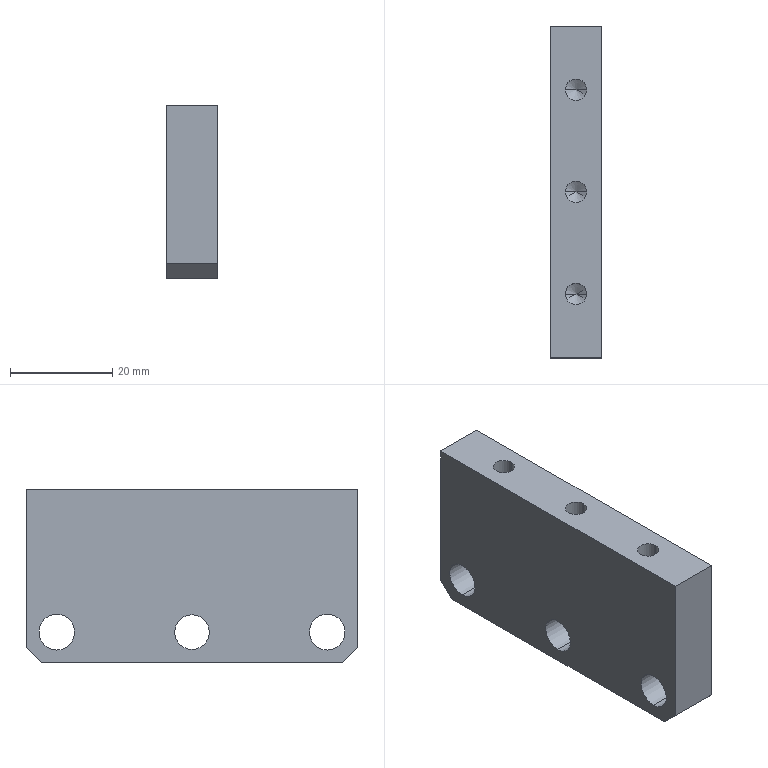Part | STEP file | A10 | 1 solid | 26 faces | box 10 x 65 x 34 mm | volume 20344 mm3 | cylinder 12 | plane 8 | cone 6 | commonest cylinder face diameters 4.2 x6 7 x4 6.8 x2